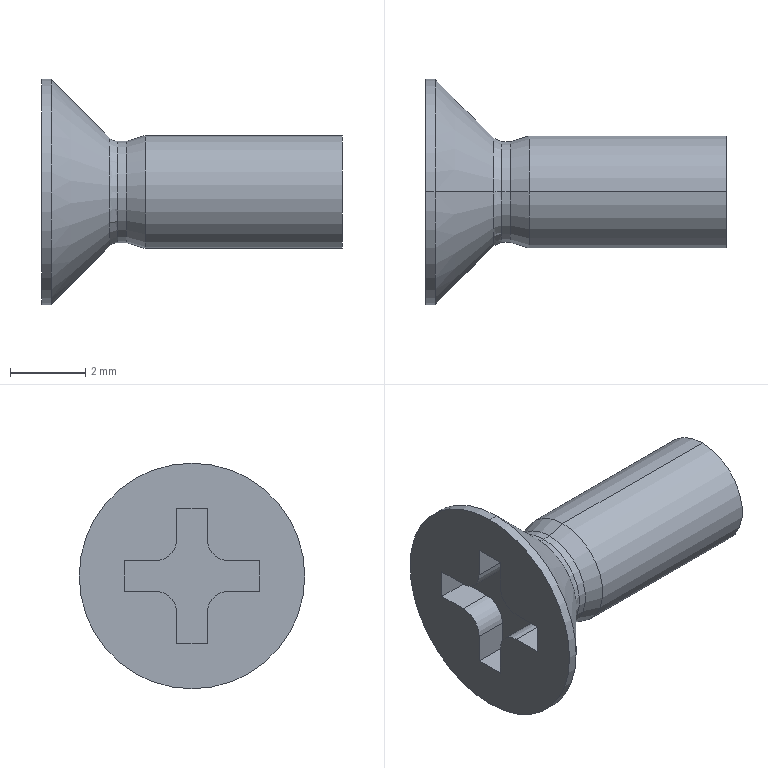Part | STEP file | 0246_020_SFBJ3-8 | 1 solid | 31 faces | box 8 x 6 x 6 mm | volume 70.323 mm3 | plane 15 | cylinder 10 | cone 4 | spline 2 | commonest cylinder face diameters 1.2 x4 2.693 x2 3 x2 6 x2